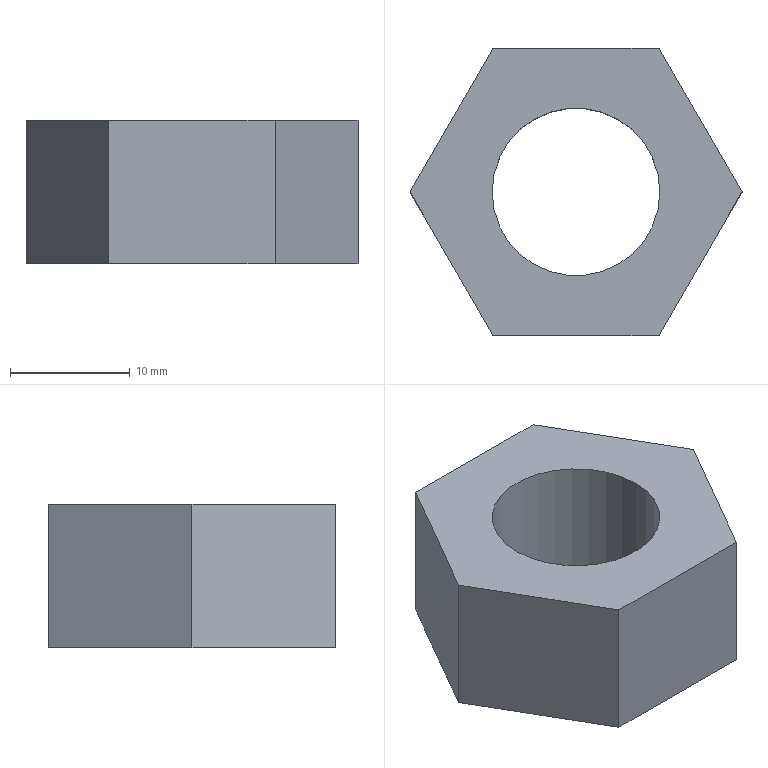Part | STEP file | Tan M16 | 1 solid | 10 faces | box 27.713 x 24 x 12 mm | volume 4139 mm3 | plane 8 | cylinder 2 | commonest cylinder face diameters 14 x2
STEP:
#1=CARTESIAN_POINT('',(0.,0.,0.));
#2=DIRECTION('',(0.,0.,1.));
#3=DIRECTION('',(1.,0.,0.));
#4=AXIS2_PLACEMENT_3D('',#1,#2,#3);
#5=CARTESIAN_POINT('',(-7.,0.,12.));
#6=VERTEX_POINT('',#5);
#7=CARTESIAN_POINT('',(-7.,0.,0.));
#8=VERTEX_POINT('',#7);
#9=CARTESIAN_POINT('',(-7.,0.,12.));
#10=DIRECTION('',(0.,0.,-1.));
#11=VECTOR('',#10,1.);
#12=LINE('',#9,#11);
#13=CARTESIAN_POINT('',(0.,0.,12.));
#14=DIRECTION('',(0.,0.,-1.));
#15=DIRECTION('',(-1.,0.,0.));
#16=AXIS2_PLACEMENT_3D('',#13,#14,#15);
#17=CYLINDRICAL_SURFACE('',#16,7.);
#18=CARTESIAN_POINT('',(6.283,0.));
#19=DIRECTION('',(0.,1.));
#20=VECTOR('',#19,1.);
#21=LINE('',#18,#20);
#22=(GEOMETRIC_REPRESENTATION_CONTEXT(2)PARAMETRIC_REPRESENTATION_CONTEXT()REPRESENTATION_CONTEXT('',''));
#23=DEFINITIONAL_REPRESENTATION('',(#21),#22);
#24=PCURVE('',#17,#23);
#25=CARTESIAN_POINT('',(0.,0.,12.));
#26=DIRECTION('',(0.,0.,-1.));
#27=DIRECTION('',(-1.,0.,0.));
#28=AXIS2_PLACEMENT_3D('',#25,#26,#27);
#29=CYLINDRICAL_SURFACE('',#28,7.);
#30=CARTESIAN_POINT('',(0.,0.));
#31=DIRECTION('',(0.,1.));
#32=VECTOR('',#31,1.);
#33=LINE('',#30,#32);
#34=(GEOMETRIC_REPRESENTATION_CONTEXT(2)PARAMETRIC_REPRESENTATION_CONTEXT()REPRESENTATION_CONTEXT('',''));
#35=DEFINITIONAL_REPRESENTATION('',(#33),#34);
#36=PCURVE('',#29,#35);
#37=SURFACE_CURVE('',#12,(#24,#36),.PCURVE_S1.);
#38=EDGE_CURVE('',#6,#8,#37,.T.);
#39=ORIENTED_EDGE('',*,*,#38,.T.);
#40=CARTESIAN_POINT('',(7.,0.,0.));
#41=VERTEX_POINT('',#40);
#42=CARTESIAN_POINT('',(0.,0.,0.));
#43=DIRECTION('',(0.,0.,1.));
#44=DIRECTION('',(1.,0.,0.));
#45=AXIS2_PLACEMENT_3D('',#42,#43,#44);
#46=CIRCLE('',#45,7.);
#47=CARTESIAN_POINT('',(9.425,12.));
#48=DIRECTION('',(-1.,0.));
#49=VECTOR('',#48,1.);
#50=LINE('',#47,#49);
#51=(GEOMETRIC_REPRESENTATION_CONTEXT(2)PARAMETRIC_REPRESENTATION_CONTEXT()REPRESENTATION_CONTEXT('',''));
#52=DEFINITIONAL_REPRESENTATION('',(#50),#51);
#53=PCURVE('',#17,#52);
#54=CARTESIAN_POINT('',(0.,0.,0.));
#55=DIRECTION('',(0.,0.,1.));
#56=DIRECTION('',(1.,0.,0.));
#57=AXIS2_PLACEMENT_3D('',#54,#55,#56);
#58=PLANE('',#57);
#59=CARTESIAN_POINT('',(0.,0.));
#60=DIRECTION('',(1.,0.));
#61=AXIS2_PLACEMENT_2D('',#59,#60);
#62=CIRCLE('',#61,7.);
#63=(GEOMETRIC_REPRESENTATION_CONTEXT(2)PARAMETRIC_REPRESENTATION_CONTEXT()REPRESENTATION_CONTEXT('',''));
#64=DEFINITIONAL_REPRESENTATION('',(#62),#63);
#65=PCURVE('',#58,#64);
#66=SURFACE_CURVE('',#46,(#53,#65),.PCURVE_S1.);
#67=EDGE_CURVE('',#8,#41,#66,.T.);
#68=ORIENTED_EDGE('',*,*,#67,.T.);
#69=CARTESIAN_POINT('',(7.,0.,12.));
#70=VERTEX_POINT('',#69);
#71=CARTESIAN_POINT('',(7.,0.,12.));
#72=DIRECTION('',(0.,0.,-1.));
#73=VECTOR('',#72,1.);
#74=LINE('',#71,#73);
#75=CARTESIAN_POINT('',(3.142,0.));
#76=DIRECTION('',(0.,1.));
#77=VECTOR('',#76,1.);
#78=LINE('',#75,#77);
#79=(GEOMETRIC_REPRESENTATION_CONTEXT(2)PARAMETRIC_REPRESENTATION_CONTEXT()REPRESENTATION_CONTEXT('',''));
#80=DEFINITIONAL_REPRESENTATION('',(#78),#79);
#81=PCURVE('',#17,#80);
#82=CARTESIAN_POINT('',(3.142,0.));
#83=DIRECTION('',(0.,1.));
#84=VECTOR('',#83,1.);
#85=LINE('',#82,#84);
#86=(GEOMETRIC_REPRESENTATION_CONTEXT(2)PARAMETRIC_REPRESENTATION_CONTEXT()REPRESENTATION_CONTEXT('',''));
#87=DEFINITIONAL_REPRESENTATION('',(#85),#86);
#88=PCURVE('',#29,#87);
#89=SURFACE_CURVE('',#74,(#81,#88),.PCURVE_S1.);
#90=EDGE_CURVE('',#70,#41,#89,.T.);
#91=ORIENTED_EDGE('',*,*,#90,.F.);
#92=CARTESIAN_POINT('',(0.,0.,12.));
#93=DIRECTION('',(0.,0.,1.));
#94=DIRECTION('',(1.,0.,0.));
#95=AXIS2_PLACEMENT_3D('',#92,#93,#94);
#96=CIRCLE('',#95,7.);
#97=CARTESIAN_POINT('',(9.425,0.));
#98=DIRECTION('',(-1.,0.));
#99=VECTOR('',#98,1.);
#100=LINE('',#97,#99);
#101=(GEOMETRIC_REPRESENTATION_CONTEXT(2)PARAMETRIC_REPRESENTATION_CONTEXT()REPRESENTATION_CONTEXT('',''));
#102=DEFINITIONAL_REPRESENTATION('',(#100),#101);
#103=PCURVE('',#17,#102);
#104=CARTESIAN_POINT('',(0.,0.,12.));
#105=DIRECTION('',(0.,0.,1.));
#106=DIRECTION('',(1.,0.,0.));
#107=AXIS2_PLACEMENT_3D('',#104,#105,#106);
#108=PLANE('',#107);
#109=CARTESIAN_POINT('',(0.,0.));
#110=DIRECTION('',(1.,0.));
#111=AXIS2_PLACEMENT_2D('',#109,#110);
#112=CIRCLE('',#111,7.);
#113=(GEOMETRIC_REPRESENTATION_CONTEXT(2)PARAMETRIC_REPRESENTATION_CONTEXT()REPRESENTATION_CONTEXT('',''));
#114=DEFINITIONAL_REPRESENTATION('',(#112),#113);
#115=PCURVE('',#108,#114);
#116=SURFACE_CURVE('',#96,(#103,#115),.PCURVE_S1.);
#117=EDGE_CURVE('',#6,#70,#116,.T.);
#118=ORIENTED_EDGE('',*,*,#117,.F.);
#119=EDGE_LOOP('',(#39,#68,#91,#118));
#120=FACE_BOUND('',#119,.F.);
#121=ADVANCED_FACE('',(#120),#17,.F.);
#122=CARTESIAN_POINT('',(6.928,-12.,12.));
#123=VERTEX_POINT('',#122);
#124=CARTESIAN_POINT('',(13.856,0.,12.));
#125=VERTEX_POINT('',#124);
#126=CARTESIAN_POINT('',(6.928,-12.,12.));
#127=DIRECTION('',(0.5,0.866,0.));
#128=VECTOR('',#127,1.);
#129=LINE('',#126,#128);
#130=CARTESIAN_POINT('',(6.928,-12.));
#131=DIRECTION('',(0.5,0.866));
#132=VECTOR('',#131,1.);
#133=LINE('',#130,#132);
#134=(GEOMETRIC_REPRESENTATION_CONTEXT(2)PARAMETRIC_REPRESENTATION_CONTEXT()REPRESENTATION_CONTEXT('',''));
#135=DEFINITIONAL_REPRESENTATION('',(#133),#134);
#136=PCURVE('',#108,#135);
#137=CARTESIAN_POINT('',(6.928,-12.,12.));
#138=DIRECTION('',(-0.866,0.5,0.));
#139=DIRECTION('',(-0.5,-0.866,0.));
#140=AXIS2_PLACEMENT_3D('',#137,#138,#139);
#141=PLANE('',#140);
#142=CARTESIAN_POINT('',(0.,0.));
#143=DIRECTION('',(-1.,0.));
#144=VECTOR('',#143,1.);
#145=LINE('',#142,#144);
#146=(GEOMETRIC_REPRESENTATION_CONTEXT(2)PARAMETRIC_REPRESENTATION_CONTEXT()REPRESENTATION_CONTEXT('',''));
#147=DEFINITIONAL_REPRESENTATION('',(#145),#146);
#148=PCURVE('',#141,#147);
#149=SURFACE_CURVE('',#129,(#136,#148),.PCURVE_S1.);
#150=EDGE_CURVE('',#123,#125,#149,.T.);
#151=ORIENTED_EDGE('',*,*,#150,.T.);
#152=CARTESIAN_POINT('',(6.928,12.,12.));
#153=VERTEX_POINT('',#152);
#154=CARTESIAN_POINT('',(13.856,0.,12.));
#155=DIRECTION('',(-0.5,0.866,0.));
#156=VECTOR('',#155,1.);
#157=LINE('',#154,#156);
#158=CARTESIAN_POINT('',(13.856,0.));
#159=DIRECTION('',(-0.5,0.866));
#160=VECTOR('',#159,1.);
#161=LINE('',#158,#160);
#162=(GEOMETRIC_REPRESENTATION_CONTEXT(2)PARAMETRIC_REPRESENTATION_CONTEXT()REPRESENTATION_CONTEXT('',''));
#163=DEFINITIONAL_REPRESENTATION('',(#161),#162);
#164=PCURVE('',#108,#163);
#165=CARTESIAN_POINT('',(13.856,0.,12.));
#166=DIRECTION('',(-0.866,-0.5,0.));
#167=DIRECTION('',(0.5,-0.866,0.));
#168=AXIS2_PLACEMENT_3D('',#165,#166,#167);
#169=PLANE('',#168);
#170=CARTESIAN_POINT('',(0.,0.));
#171=DIRECTION('',(-1.,0.));
#172=VECTOR('',#171,1.);
#173=LINE('',#170,#172);
#174=(GEOMETRIC_REPRESENTATION_CONTEXT(2)PARAMETRIC_REPRESENTATION_CONTEXT()REPRESENTATION_CONTEXT('',''));
#175=DEFINITIONAL_REPRESENTATION('',(#173),#174);
#176=PCURVE('',#169,#175);
#177=SURFACE_CURVE('',#157,(#164,#176),.PCURVE_S1.);
#178=EDGE_CURVE('',#125,#153,#177,.T.);
#179=ORIENTED_EDGE('',*,*,#178,.T.);
#180=CARTESIAN_POINT('',(-6.928,12.,12.));
#181=VERTEX_POINT('',#180);
#182=CARTESIAN_POINT('',(6.928,12.,12.));
#183=DIRECTION('',(-1.,0.,0.));
#184=VECTOR('',#183,1.);
#185=LINE('',#182,#184);
#186=CARTESIAN_POINT('',(6.928,12.));
#187=DIRECTION('',(-1.,0.));
#188=VECTOR('',#187,1.);
#189=LINE('',#186,#188);
#190=(GEOMETRIC_REPRESENTATION_CONTEXT(2)PARAMETRIC_REPRESENTATION_CONTEXT()REPRESENTATION_CONTEXT('',''));
#191=DEFINITIONAL_REPRESENTATION('',(#189),#190);
#192=PCURVE('',#108,#191);
#193=CARTESIAN_POINT('',(6.928,12.,12.));
#194=DIRECTION('',(0.,-1.,0.));
#195=DIRECTION('',(0.,0.,-1.));
#196=AXIS2_PLACEMENT_3D('',#193,#194,#195);
#197=PLANE('',#196);
#198=CARTESIAN_POINT('',(0.,0.));
#199=DIRECTION('',(0.,-1.));
#200=VECTOR('',#199,1.);
#201=LINE('',#198,#200);
#202=(GEOMETRIC_REPRESENTATION_CONTEXT(2)PARAMETRIC_REPRESENTATION_CONTEXT()REPRESENTATION_CONTEXT('',''));
#203=DEFINITIONAL_REPRESENTATION('',(#201),#202);
#204=PCURVE('',#197,#203);
#205=SURFACE_CURVE('',#185,(#192,#204),.PCURVE_S1.);
#206=EDGE_CURVE('',#153,#181,#205,.T.);
#207=ORIENTED_EDGE('',*,*,#206,.T.);
#208=CARTESIAN_POINT('',(-13.856,0.,12.));
#209=VERTEX_POINT('',#208);
#210=CARTESIAN_POINT('',(-6.928,12.,12.));
#211=DIRECTION('',(-0.5,-0.866,0.));
#212=VECTOR('',#211,1.);
#213=LINE('',#210,#212);
#214=CARTESIAN_POINT('',(-6.928,12.));
#215=DIRECTION('',(-0.5,-0.866));
#216=VECTOR('',#215,1.);
#217=LINE('',#214,#216);
#218=(GEOMETRIC_REPRESENTATION_CONTEXT(2)PARAMETRIC_REPRESENTATION_CONTEXT()REPRESENTATION_CONTEXT('',''));
#219=DEFINITIONAL_REPRESENTATION('',(#217),#218);
#220=PCURVE('',#108,#219);
#221=CARTESIAN_POINT('',(-6.928,12.,12.));
#222=DIRECTION('',(0.866,-0.5,0.));
#223=DIRECTION('',(0.5,0.866,0.));
#224=AXIS2_PLACEMENT_3D('',#221,#222,#223);
#225=PLANE('',#224);
#226=CARTESIAN_POINT('',(0.,0.));
#227=DIRECTION('',(-1.,0.));
#228=VECTOR('',#227,1.);
#229=LINE('',#226,#228);
#230=(GEOMETRIC_REPRESENTATION_CONTEXT(2)PARAMETRIC_REPRESENTATION_CONTEXT()REPRESENTATION_CONTEXT('',''));
#231=DEFINITIONAL_REPRESENTATION('',(#229),#230);
#232=PCURVE('',#225,#231);
#233=SURFACE_CURVE('',#213,(#220,#232),.PCURVE_S1.);
#234=EDGE_CURVE('',#181,#209,#233,.T.);
#235=ORIENTED_EDGE('',*,*,#234,.T.);
#236=CARTESIAN_POINT('',(-6.928,-12.,12.));
#237=VERTEX_POINT('',#236);
#238=CARTESIAN_POINT('',(-13.856,0.,12.));
#239=DIRECTION('',(0.5,-0.866,0.));
#240=VECTOR('',#239,1.);
#241=LINE('',#238,#240);
#242=CARTESIAN_POINT('',(-13.856,0.));
#243=DIRECTION('',(0.5,-0.866));
#244=VECTOR('',#243,1.);
#245=LINE('',#242,#244);
#246=(GEOMETRIC_REPRESENTATION_CONTEXT(2)PARAMETRIC_REPRESENTATION_CONTEXT()REPRESENTATION_CONTEXT('',''));
#247=DEFINITIONAL_REPRESENTATION('',(#245),#246);
#248=PCURVE('',#108,#247);
#249=CARTESIAN_POINT('',(-13.856,0.,12.));
#250=DIRECTION('',(0.866,0.5,0.));
#251=DIRECTION('',(-0.5,0.866,0.));
#252=AXIS2_PLACEMENT_3D('',#249,#250,#251);
#253=PLANE('',#252);
#254=CARTESIAN_POINT('',(0.,0.));
#255=DIRECTION('',(-1.,0.));
#256=VECTOR('',#255,1.);
#257=LINE('',#254,#256);
#258=(GEOMETRIC_REPRESENTATION_CONTEXT(2)PARAMETRIC_REPRESENTATION_CONTEXT()REPRESENTATION_CONTEXT('',''));
#259=DEFINITIONAL_REPRESENTATION('',(#257),#258);
#260=PCURVE('',#253,#259);
#261=SURFACE_CURVE('',#241,(#248,#260),.PCURVE_S1.);
#262=EDGE_CURVE('',#209,#237,#261,.T.);
#263=ORIENTED_EDGE('',*,*,#262,.T.);
#264=CARTESIAN_POINT('',(-6.928,-12.,12.));
#265=DIRECTION('',(1.,0.,0.));
#266=VECTOR('',#265,1.);
#267=LINE('',#264,#266);
#268=CARTESIAN_POINT('',(-6.928,-12.));
#269=DIRECTION('',(1.,0.));
#270=VECTOR('',#269,1.);
#271=LINE('',#268,#270);
#272=(GEOMETRIC_REPRESENTATION_CONTEXT(2)PARAMETRIC_REPRESENTATION_CONTEXT()REPRESENTATION_CONTEXT('',''));
#273=DEFINITIONAL_REPRESENTATION('',(#271),#272);
#274=PCURVE('',#108,#273);
#275=CARTESIAN_POINT('',(-6.928,-12.,12.));
#276=DIRECTION('',(0.,1.,0.));
#277=DIRECTION('',(-1.,0.,0.));
#278=AXIS2_PLACEMENT_3D('',#275,#276,#277);
#279=PLANE('',#278);
#280=CARTESIAN_POINT('',(0.,0.));
#281=DIRECTION('',(-1.,0.));
#282=VECTOR('',#281,1.);
#283=LINE('',#280,#282);
#284=(GEOMETRIC_REPRESENTATION_CONTEXT(2)PARAMETRIC_REPRESENTATION_CONTEXT()REPRESENTATION_CONTEXT('',''));
#285=DEFINITIONAL_REPRESENTATION('',(#283),#284);
#286=PCURVE('',#279,#285);
#287=SURFACE_CURVE('',#267,(#274,#286),.PCURVE_S1.);
#288=EDGE_CURVE('',#237,#123,#287,.T.);
#289=ORIENTED_EDGE('',*,*,#288,.T.);
#290=EDGE_LOOP('',(#151,#179,#207,#235,#263,#289));
#291=FACE_BOUND('',#290,.T.);
#292=ORIENTED_EDGE('',*,*,#117,.F.);
#293=CARTESIAN_POINT('',(0.,0.,12.));
#294=DIRECTION('',(0.,0.,1.));
#295=DIRECTION('',(1.,0.,0.));
#296=AXIS2_PLACEMENT_3D('',#293,#294,#295);
#297=CIRCLE('',#296,7.);
#298=CARTESIAN_POINT('',(0.,0.));
#299=DIRECTION('',(1.,0.));
#300=AXIS2_PLACEMENT_2D('',#298,#299);
#301=CIRCLE('',#300,7.);
#302=(GEOMETRIC_REPRESENTATION_CONTEXT(2)PARAMETRIC_REPRESENTATION_CONTEXT()REPRESENTATION_CONTEXT('',''));
#303=DEFINITIONAL_REPRESENTATION('',(#301),#302);
#304=PCURVE('',#108,#303);
#305=CARTESIAN_POINT('',(3.142,0.));
#306=DIRECTION('',(-1.,0.));
#307=VECTOR('',#306,1.);
#308=LINE('',#305,#307);
#309=(GEOMETRIC_REPRESENTATION_CONTEXT(2)PARAMETRIC_REPRESENTATION_CONTEXT()REPRESENTATION_CONTEXT('',''));
#310=DEFINITIONAL_REPRESENTATION('',(#308),#309);
#311=PCURVE('',#29,#310);
#312=SURFACE_CURVE('',#297,(#304,#311),.PCURVE_S1.);
#313=EDGE_CURVE('',#70,#6,#312,.T.);
#314=ORIENTED_EDGE('',*,*,#313,.F.);
#315=EDGE_LOOP('',(#292,#314));
#316=FACE_BOUND('',#315,.T.);
#317=ADVANCED_FACE('',(#291,#316),#108,.T.);
#318=CARTESIAN_POINT('',(6.928,-12.,0.));
#319=VERTEX_POINT('',#318);
#320=CARTESIAN_POINT('',(13.856,0.,0.));
#321=VERTEX_POINT('',#320);
#322=CARTESIAN_POINT('',(6.928,-12.,0.));
#323=DIRECTION('',(0.5,0.866,0.));
#324=VECTOR('',#323,1.);
#325=LINE('',#322,#324);
#326=CARTESIAN_POINT('',(6.928,-12.));
#327=DIRECTION('',(0.5,0.866));
#328=VECTOR('',#327,1.);
#329=LINE('',#326,#328);
#330=(GEOMETRIC_REPRESENTATION_CONTEXT(2)PARAMETRIC_REPRESENTATION_CONTEXT()REPRESENTATION_CONTEXT('',''));
#331=DEFINITIONAL_REPRESENTATION('',(#329),#330);
#332=PCURVE('',#58,#331);
#333=CARTESIAN_POINT('',(0.,-12.));
#334=DIRECTION('',(-1.,0.));
#335=VECTOR('',#334,1.);
#336=LINE('',#333,#335);
#337=(GEOMETRIC_REPRESENTATION_CONTEXT(2)PARAMETRIC_REPRESENTATION_CONTEXT()REPRESENTATION_CONTEXT('',''));
#338=DEFINITIONAL_REPRESENTATION('',(#336),#337);
#339=PCURVE('',#141,#338);
#340=SURFACE_CURVE('',#325,(#332,#339),.PCURVE_S1.);
#341=EDGE_CURVE('',#319,#321,#340,.T.);
#342=ORIENTED_EDGE('',*,*,#341,.F.);
#343=CARTESIAN_POINT('',(-6.928,-12.,0.));
#344=VERTEX_POINT('',#343);
#345=CARTESIAN_POINT('',(-6.928,-12.,0.));
#346=DIRECTION('',(1.,0.,0.));
#347=VECTOR('',#346,1.);
#348=LINE('',#345,#347);
#349=CARTESIAN_POINT('',(-6.928,-12.));
#350=DIRECTION('',(1.,0.));
#351=VECTOR('',#350,1.);
#352=LINE('',#349,#351);
#353=(GEOMETRIC_REPRESENTATION_CONTEXT(2)PARAMETRIC_REPRESENTATION_CONTEXT()REPRESENTATION_CONTEXT('',''));
#354=DEFINITIONAL_REPRESENTATION('',(#352),#353);
#355=PCURVE('',#58,#354);
#356=CARTESIAN_POINT('',(0.,-12.));
#357=DIRECTION('',(-1.,0.));
#358=VECTOR('',#357,1.);
#359=LINE('',#356,#358);
#360=(GEOMETRIC_REPRESENTATION_CONTEXT(2)PARAMETRIC_REPRESENTATION_CONTEXT()REPRESENTATION_CONTEXT('',''));
#361=DEFINITIONAL_REPRESENTATION('',(#359),#360);
#362=PCURVE('',#279,#361);
#363=SURFACE_CURVE('',#348,(#355,#362),.PCURVE_S1.);
#364=EDGE_CURVE('',#344,#319,#363,.T.);
#365=ORIENTED_EDGE('',*,*,#364,.F.);
#366=CARTESIAN_POINT('',(-13.856,0.,0.));
#367=VERTEX_POINT('',#366);
#368=CARTESIAN_POINT('',(-13.856,0.,0.));
#369=DIRECTION('',(0.5,-0.866,0.));
#370=VECTOR('',#369,1.);
#371=LINE('',#368,#370);
#372=CARTESIAN_POINT('',(-13.856,0.));
#373=DIRECTION('',(0.5,-0.866));
#374=VECTOR('',#373,1.);
#375=LINE('',#372,#374);
#376=(GEOMETRIC_REPRESENTATION_CONTEXT(2)PARAMETRIC_REPRESENTATION_CONTEXT()REPRESENTATION_CONTEXT('',''));
#377=DEFINITIONAL_REPRESENTATION('',(#375),#376);
#378=PCURVE('',#58,#377);
#379=CARTESIAN_POINT('',(0.,-12.));
#380=DIRECTION('',(-1.,0.));
#381=VECTOR('',#380,1.);
#382=LINE('',#379,#381);
#383=(GEOMETRIC_REPRESENTATION_CONTEXT(2)PARAMETRIC_REPRESENTATION_CONTEXT()REPRESENTATION_CONTEXT('',''));
#384=DEFINITIONAL_REPRESENTATION('',(#382),#383);
#385=PCURVE('',#253,#384);
#386=SURFACE_CURVE('',#371,(#378,#385),.PCURVE_S1.);
#387=EDGE_CURVE('',#367,#344,#386,.T.);
#388=ORIENTED_EDGE('',*,*,#387,.F.);
#389=CARTESIAN_POINT('',(-6.928,12.,0.));
#390=VERTEX_POINT('',#389);
#391=CARTESIAN_POINT('',(-6.928,12.,0.));
#392=DIRECTION('',(-0.5,-0.866,0.));
#393=VECTOR('',#392,1.);
#394=LINE('',#391,#393);
#395=CARTESIAN_POINT('',(-6.928,12.));
#396=DIRECTION('',(-0.5,-0.866));
#397=VECTOR('',#396,1.);
#398=LINE('',#395,#397);
#399=(GEOMETRIC_REPRESENTATION_CONTEXT(2)PARAMETRIC_REPRESENTATION_CONTEXT()REPRESENTATION_CONTEXT('',''));
#400=DEFINITIONAL_REPRESENTATION('',(#398),#399);
#401=PCURVE('',#58,#400);
#402=CARTESIAN_POINT('',(0.,-12.));
#403=DIRECTION('',(-1.,0.));
#404=VECTOR('',#403,1.);
#405=LINE('',#402,#404);
#406=(GEOMETRIC_REPRESENTATION_CONTEXT(2)PARAMETRIC_REPRESENTATION_CONTEXT()REPRESENTATION_CONTEXT('',''));
#407=DEFINITIONAL_REPRESENTATION('',(#405),#406);
#408=PCURVE('',#225,#407);
#409=SURFACE_CURVE('',#394,(#401,#408),.PCURVE_S1.);
#410=EDGE_CURVE('',#390,#367,#409,.T.);
#411=ORIENTED_EDGE('',*,*,#410,.F.);
#412=CARTESIAN_POINT('',(6.928,12.,0.));
#413=VERTEX_POINT('',#412);
#414=CARTESIAN_POINT('',(6.928,12.,0.));
#415=DIRECTION('',(-1.,0.,0.));
#416=VECTOR('',#415,1.);
#417=LINE('',#414,#416);
#418=CARTESIAN_POINT('',(6.928,12.));
#419=DIRECTION('',(-1.,0.));
#420=VECTOR('',#419,1.);
#421=LINE('',#418,#420);
#422=(GEOMETRIC_REPRESENTATION_CONTEXT(2)PARAMETRIC_REPRESENTATION_CONTEXT()REPRESENTATION_CONTEXT('',''));
#423=DEFINITIONAL_REPRESENTATION('',(#421),#422);
#424=PCURVE('',#58,#423);
#425=CARTESIAN_POINT('',(12.,0.));
#426=DIRECTION('',(0.,-1.));
#427=VECTOR('',#426,1.);
#428=LINE('',#425,#427);
#429=(GEOMETRIC_REPRESENTATION_CONTEXT(2)PARAMETRIC_REPRESENTATION_CONTEXT()REPRESENTATION_CONTEXT('',''));
#430=DEFINITIONAL_REPRESENTATION('',(#428),#429);
#431=PCURVE('',#197,#430);
#432=SURFACE_CURVE('',#417,(#424,#431),.PCURVE_S1.);
#433=EDGE_CURVE('',#413,#390,#432,.T.);
#434=ORIENTED_EDGE('',*,*,#433,.F.);
#435=CARTESIAN_POINT('',(13.856,0.,0.));
#436=DIRECTION('',(-0.5,0.866,0.));
#437=VECTOR('',#436,1.);
#438=LINE('',#435,#437);
#439=CARTESIAN_POINT('',(13.856,0.));
#440=DIRECTION('',(-0.5,0.866));
#441=VECTOR('',#440,1.);
#442=LINE('',#439,#441);
#443=(GEOMETRIC_REPRESENTATION_CONTEXT(2)PARAMETRIC_REPRESENTATION_CONTEXT()REPRESENTATION_CONTEXT('',''));
#444=DEFINITIONAL_REPRESENTATION('',(#442),#443);
#445=PCURVE('',#58,#444);
#446=CARTESIAN_POINT('',(0.,-12.));
#447=DIRECTION('',(-1.,0.));
#448=VECTOR('',#447,1.);
#449=LINE('',#446,#448);
#450=(GEOMETRIC_REPRESENTATION_CONTEXT(2)PARAMETRIC_REPRESENTATION_CONTEXT()REPRESENTATION_CONTEXT('',''));
#451=DEFINITIONAL_REPRESENTATION('',(#449),#450);
#452=PCURVE('',#169,#451);
#453=SURFACE_CURVE('',#438,(#445,#452),.PCURVE_S1.);
#454=EDGE_CURVE('',#321,#413,#453,.T.);
#455=ORIENTED_EDGE('',*,*,#454,.F.);
#456=EDGE_LOOP('',(#342,#365,#388,#411,#434,#455));
#457=FACE_BOUND('',#456,.T.);
#458=ORIENTED_EDGE('',*,*,#67,.T.);
#459=CARTESIAN_POINT('',(0.,0.,0.));
#460=DIRECTION('',(0.,0.,1.));
#461=DIRECTION('',(1.,0.,0.));
#462=AXIS2_PLACEMENT_3D('',#459,#460,#461);
#463=CIRCLE('',#462,7.);
#464=CARTESIAN_POINT('',(0.,0.));
#465=DIRECTION('',(1.,0.));
#466=AXIS2_PLACEMENT_2D('',#464,#465);
#467=CIRCLE('',#466,7.);
#468=(GEOMETRIC_REPRESENTATION_CONTEXT(2)PARAMETRIC_REPRESENTATION_CONTEXT()REPRESENTATION_CONTEXT('',''));
#469=DEFINITIONAL_REPRESENTATION('',(#467),#468);
#470=PCURVE('',#58,#469);
#471=CARTESIAN_POINT('',(3.142,12.));
#472=DIRECTION('',(-1.,0.));
#473=VECTOR('',#472,1.);
#474=LINE('',#471,#473);
#475=(GEOMETRIC_REPRESENTATION_CONTEXT(2)PARAMETRIC_REPRESENTATION_CONTEXT()REPRESENTATION_CONTEXT('',''));
#476=DEFINITIONAL_REPRESENTATION('',(#474),#475);
#477=PCURVE('',#29,#476);
#478=SURFACE_CURVE('',#463,(#470,#477),.PCURVE_S1.);
#479=EDGE_CURVE('',#41,#8,#478,.T.);
#480=ORIENTED_EDGE('',*,*,#479,.T.);
#481=EDGE_LOOP('',(#458,#480));
#482=FACE_BOUND('',#481,.T.);
#483=ADVANCED_FACE('',(#457,#482),#58,.F.);
#484=ORIENTED_EDGE('',*,*,#341,.T.);
#485=CARTESIAN_POINT('',(13.856,0.,12.));
#486=DIRECTION('',(0.,0.,-1.));
#487=VECTOR('',#486,1.);
#488=LINE('',#485,#487);
#489=CARTESIAN_POINT('',(-13.856,0.));
#490=DIRECTION('',(0.,-1.));
#491=VECTOR('',#490,1.);
#492=LINE('',#489,#491);
#493=(GEOMETRIC_REPRESENTATION_CONTEXT(2)PARAMETRIC_REPRESENTATION_CONTEXT()REPRESENTATION_CONTEXT('',''));
#494=DEFINITIONAL_REPRESENTATION('',(#492),#493);
#495=PCURVE('',#141,#494);
#496=CARTESIAN_POINT('',(0.,0.));
#497=DIRECTION('',(0.,-1.));
#498=VECTOR('',#497,1.);
#499=LINE('',#496,#498);
#500=(GEOMETRIC_REPRESENTATION_CONTEXT(2)PARAMETRIC_REPRESENTATION_CONTEXT()REPRESENTATION_CONTEXT('',''));
#501=DEFINITIONAL_REPRESENTATION('',(#499),#500);
#502=PCURVE('',#169,#501);
#503=SURFACE_CURVE('',#488,(#495,#502),.PCURVE_S1.);
#504=EDGE_CURVE('',#125,#321,#503,.T.);
#505=ORIENTED_EDGE('',*,*,#504,.F.);
#506=ORIENTED_EDGE('',*,*,#150,.F.);
#507=CARTESIAN_POINT('',(6.928,-12.,12.));
#508=DIRECTION('',(0.,0.,-1.));
#509=VECTOR('',#508,1.);
#510=LINE('',#507,#509);
#511=CARTESIAN_POINT('',(0.,0.));
#512=DIRECTION('',(0.,-1.));
#513=VECTOR('',#512,1.);
#514=LINE('',#511,#513);
#515=(GEOMETRIC_REPRESENTATION_CONTEXT(2)PARAMETRIC_REPRESENTATION_CONTEXT()REPRESENTATION_CONTEXT('',''));
#516=DEFINITIONAL_REPRESENTATION('',(#514),#515);
#517=PCURVE('',#141,#516);
#518=CARTESIAN_POINT('',(-13.856,0.));
#519=DIRECTION('',(0.,-1.));
#520=VECTOR('',#519,1.);
#521=LINE('',#518,#520);
#522=(GEOMETRIC_REPRESENTATION_CONTEXT(2)PARAMETRIC_REPRESENTATION_CONTEXT()REPRESENTATION_CONTEXT('',''));
#523=DEFINITIONAL_REPRESENTATION('',(#521),#522);
#524=PCURVE('',#279,#523);
#525=SURFACE_CURVE('',#510,(#517,#524),.PCURVE_S1.);
#526=EDGE_CURVE('',#123,#319,#525,.T.);
#527=ORIENTED_EDGE('',*,*,#526,.T.);
#528=EDGE_LOOP('',(#484,#505,#506,#527));
#529=FACE_BOUND('',#528,.T.);
#530=ADVANCED_FACE('',(#529),#141,.F.);
#531=ORIENTED_EDGE('',*,*,#454,.T.);
#532=CARTESIAN_POINT('',(6.928,12.,12.));
#533=DIRECTION('',(0.,0.,-1.));
#534=VECTOR('',#533,1.);
#535=LINE('',#532,#534);
#536=CARTESIAN_POINT('',(-13.856,0.));
#537=DIRECTION('',(0.,-1.));
#538=VECTOR('',#537,1.);
#539=LINE('',#536,#538);
#540=(GEOMETRIC_REPRESENTATION_CONTEXT(2)PARAMETRIC_REPRESENTATION_CONTEXT()REPRESENTATION_CONTEXT('',''));
#541=DEFINITIONAL_REPRESENTATION('',(#539),#540);
#542=PCURVE('',#169,#541);
#543=CARTESIAN_POINT('',(0.,0.));
#544=DIRECTION('',(1.,0.));
#545=VECTOR('',#544,1.);
#546=LINE('',#543,#545);
#547=(GEOMETRIC_REPRESENTATION_CONTEXT(2)PARAMETRIC_REPRESENTATION_CONTEXT()REPRESENTATION_CONTEXT('',''));
#548=DEFINITIONAL_REPRESENTATION('',(#546),#547);
#549=PCURVE('',#197,#548);
#550=SURFACE_CURVE('',#535,(#542,#549),.PCURVE_S1.);
#551=EDGE_CURVE('',#153,#413,#550,.T.);
#552=ORIENTED_EDGE('',*,*,#551,.F.);
#553=ORIENTED_EDGE('',*,*,#178,.F.);
#554=ORIENTED_EDGE('',*,*,#504,.T.);
#555=EDGE_LOOP('',(#531,#552,#553,#554));
#556=FACE_BOUND('',#555,.T.);
#557=ADVANCED_FACE('',(#556),#169,.F.);
#558=ORIENTED_EDGE('',*,*,#433,.T.);
#559=CARTESIAN_POINT('',(-6.928,12.,12.));
#560=DIRECTION('',(0.,0.,-1.));
#561=VECTOR('',#560,1.);
#562=LINE('',#559,#561);
#563=CARTESIAN_POINT('',(0.,-13.856));
#564=DIRECTION('',(1.,0.));
#565=VECTOR('',#564,1.);
#566=LINE('',#563,#565);
#567=(GEOMETRIC_REPRESENTATION_CONTEXT(2)PARAMETRIC_REPRESENTATION_CONTEXT()REPRESENTATION_CONTEXT('',''));
#568=DEFINITIONAL_REPRESENTATION('',(#566),#567);
#569=PCURVE('',#197,#568);
#570=CARTESIAN_POINT('',(0.,0.));
#571=DIRECTION('',(0.,-1.));
#572=VECTOR('',#571,1.);
#573=LINE('',#570,#572);
#574=(GEOMETRIC_REPRESENTATION_CONTEXT(2)PARAMETRIC_REPRESENTATION_CONTEXT()REPRESENTATION_CONTEXT('',''));
#575=DEFINITIONAL_REPRESENTATION('',(#573),#574);
#576=PCURVE('',#225,#575);
#577=SURFACE_CURVE('',#562,(#569,#576),.PCURVE_S1.);
#578=EDGE_CURVE('',#181,#390,#577,.T.);
#579=ORIENTED_EDGE('',*,*,#578,.F.);
#580=ORIENTED_EDGE('',*,*,#206,.F.);
#581=ORIENTED_EDGE('',*,*,#551,.T.);
#582=EDGE_LOOP('',(#558,#579,#580,#581));
#583=FACE_BOUND('',#582,.T.);
#584=ADVANCED_FACE('',(#583),#197,.F.);
#585=ORIENTED_EDGE('',*,*,#410,.T.);
#586=CARTESIAN_POINT('',(-13.856,0.,12.));
#587=DIRECTION('',(0.,0.,-1.));
#588=VECTOR('',#587,1.);
#589=LINE('',#586,#588);
#590=CARTESIAN_POINT('',(-13.856,0.));
#591=DIRECTION('',(0.,-1.));
#592=VECTOR('',#591,1.);
#593=LINE('',#590,#592);
#594=(GEOMETRIC_REPRESENTATION_CONTEXT(2)PARAMETRIC_REPRESENTATION_CONTEXT()REPRESENTATION_CONTEXT('',''));
#595=DEFINITIONAL_REPRESENTATION('',(#593),#594);
#596=PCURVE('',#225,#595);
#597=CARTESIAN_POINT('',(0.,0.));
#598=DIRECTION('',(0.,-1.));
#599=VECTOR('',#598,1.);
#600=LINE('',#597,#599);
#601=(GEOMETRIC_REPRESENTATION_CONTEXT(2)PARAMETRIC_REPRESENTATION_CONTEXT()REPRESENTATION_CONTEXT('',''));
#602=DEFINITIONAL_REPRESENTATION('',(#600),#601);
#603=PCURVE('',#253,#602);
#604=SURFACE_CURVE('',#589,(#596,#603),.PCURVE_S1.);
#605=EDGE_CURVE('',#209,#367,#604,.T.);
#606=ORIENTED_EDGE('',*,*,#605,.F.);
#607=ORIENTED_EDGE('',*,*,#234,.F.);
#608=ORIENTED_EDGE('',*,*,#578,.T.);
#609=EDGE_LOOP('',(#585,#606,#607,#608));
#610=FACE_BOUND('',#609,.T.);
#611=ADVANCED_FACE('',(#610),#225,.F.);
#612=ORIENTED_EDGE('',*,*,#387,.T.);
#613=CARTESIAN_POINT('',(-6.928,-12.,12.));
#614=DIRECTION('',(0.,0.,-1.));
#615=VECTOR('',#614,1.);
#616=LINE('',#613,#615);
#617=CARTESIAN_POINT('',(-13.856,0.));
#618=DIRECTION('',(0.,-1.));
#619=VECTOR('',#618,1.);
#620=LINE('',#617,#619);
#621=(GEOMETRIC_REPRESENTATION_CONTEXT(2)PARAMETRIC_REPRESENTATION_CONTEXT()REPRESENTATION_CONTEXT('',''));
#622=DEFINITIONAL_REPRESENTATION('',(#620),#621);
#623=PCURVE('',#253,#622);
#624=CARTESIAN_POINT('',(0.,0.));
#625=DIRECTION('',(0.,-1.));
#626=VECTOR('',#625,1.);
#627=LINE('',#624,#626);
#628=(GEOMETRIC_REPRESENTATION_CONTEXT(2)PARAMETRIC_REPRESENTATION_CONTEXT()REPRESENTATION_CONTEXT('',''));
#629=DEFINITIONAL_REPRESENTATION('',(#627),#628);
#630=PCURVE('',#279,#629);
#631=SURFACE_CURVE('',#616,(#623,#630),.PCURVE_S1.);
#632=EDGE_CURVE('',#237,#344,#631,.T.);
#633=ORIENTED_EDGE('',*,*,#632,.F.);
#634=ORIENTED_EDGE('',*,*,#262,.F.);
#635=ORIENTED_EDGE('',*,*,#605,.T.);
#636=EDGE_LOOP('',(#612,#633,#634,#635));
#637=FACE_BOUND('',#636,.T.);
#638=ADVANCED_FACE('',(#637),#253,.F.);
#639=ORIENTED_EDGE('',*,*,#364,.T.);
#640=ORIENTED_EDGE('',*,*,#526,.F.);
#641=ORIENTED_EDGE('',*,*,#288,.F.);
#642=ORIENTED_EDGE('',*,*,#632,.T.);
#643=EDGE_LOOP('',(#639,#640,#641,#642));
#644=FACE_BOUND('',#643,.T.);
#645=ADVANCED_FACE('',(#644),#279,.F.);
#646=ORIENTED_EDGE('',*,*,#479,.T.);
#647=ORIENTED_EDGE('',*,*,#38,.F.);
#648=ORIENTED_EDGE('',*,*,#313,.F.);
#649=ORIENTED_EDGE('',*,*,#90,.T.);
#650=EDGE_LOOP('',(#646,#647,#648,#649));
#651=FACE_BOUND('',#650,.F.);
#652=ADVANCED_FACE('',(#651),#29,.F.);
#653=CLOSED_SHELL('',(#121,#317,#483,#530,#557,#584,#611,#638,#645,#652));
#654=MANIFOLD_SOLID_BREP('',#653);
#655=(LENGTH_UNIT()NAMED_UNIT(*)SI_UNIT(.MILLI.,.METRE.));
#656=UNCERTAINTY_MEASURE_WITH_UNIT(LENGTH_MEASURE(0.0000001),#655,'','');
#657=(NAMED_UNIT(*)PLANE_ANGLE_UNIT()SI_UNIT($,.RADIAN.));
#658=(NAMED_UNIT(*)SI_UNIT($,.STERADIAN.)SOLID_ANGLE_UNIT());
#659=(GEOMETRIC_REPRESENTATION_CONTEXT(3)GLOBAL_UNCERTAINTY_ASSIGNED_CONTEXT((#656))GLOBAL_UNIT_ASSIGNED_CONTEXT((#655,#657,#658))REPRESENTATION_CONTEXT('',''));
#660=ADVANCED_BREP_SHAPE_REPRESENTATION('',(#4,#654),#659);